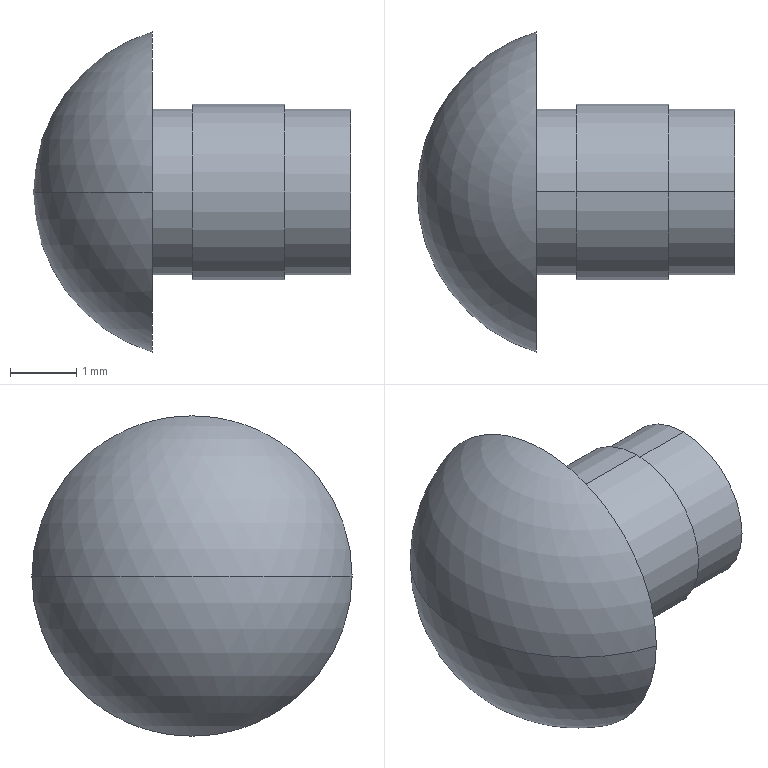Part | SolidWorks | features Boss 1, RevCut 1, Revolution 1 | 1 solid | 12 faces | box 4.8 x 4.84 x 4.84 mm | volume 35.188 mm3 | cylinder 6 | plane 4 | sphere 2 | commonest cylinder face diameters 2.5 x4 2.65 x2
STEP:
#1=CARTESIAN_POINT('',(3.8,0.,-1.25));
#2=VERTEX_POINT('',#1);
#3=CARTESIAN_POINT('',(3.8,0.,1.25));
#4=VERTEX_POINT('',#3);
#5=CARTESIAN_POINT('',(3.8,0.,0.));
#6=DIRECTION('',(1.,0.,0.));
#7=DIRECTION('',(0.,0.,-1.));
#8=AXIS2_PLACEMENT_3D('',#5,#6,#7);
#9=CIRCLE('',#8,1.25);
#10=EDGE_CURVE('',#2,#4,#9,.T.);
#11=ORIENTED_EDGE('',*,*,#10,.T.);
#12=CARTESIAN_POINT('',(4.8,0.,1.25));
#13=VERTEX_POINT('',#12);
#14=CARTESIAN_POINT('',(0.8134,0.,1.25));
#15=DIRECTION('',(1.,0.,0.));
#16=VECTOR('',#15,1000.);
#17=LINE('',#14,#16);
#18=EDGE_CURVE('',#4,#13,#17,.T.);
#19=ORIENTED_EDGE('',*,*,#18,.T.);
#20=CARTESIAN_POINT('',(4.8,0.,-1.25));
#21=VERTEX_POINT('',#20);
#22=CARTESIAN_POINT('',(4.8,0.,0.));
#23=DIRECTION('',(1.,0.,0.));
#24=DIRECTION('',(0.,0.,-1.));
#25=AXIS2_PLACEMENT_3D('',#22,#23,#24);
#26=CIRCLE('',#25,1.25);
#27=EDGE_CURVE('',#21,#13,#26,.T.);
#28=ORIENTED_EDGE('',*,*,#27,.F.);
#29=CARTESIAN_POINT('',(0.8134,0.,-1.25));
#30=DIRECTION('',(1.,0.,0.));
#31=VECTOR('',#30,1000.);
#32=LINE('',#29,#31);
#33=EDGE_CURVE('',#2,#21,#32,.T.);
#34=ORIENTED_EDGE('',*,*,#33,.F.);
#35=EDGE_LOOP('',(#11,#19,#28,#34));
#36=FACE_OUTER_BOUND('',#35,.T.);
#37=CARTESIAN_POINT('',(0.8134,0.,0.));
#38=DIRECTION('',(1.,0.,0.));
#39=DIRECTION('',(0.,0.,-1.));
#40=AXIS2_PLACEMENT_3D('',#37,#38,#39);
#41=CYLINDRICAL_SURFACE('',#40,1.25);
#42=ADVANCED_FACE('',(#36),#41,.T.);
#43=CARTESIAN_POINT('',(2.4,0.,-1.325));
#44=VERTEX_POINT('',#43);
#45=CARTESIAN_POINT('',(2.4,0.,1.325));
#46=VERTEX_POINT('',#45);
#47=CARTESIAN_POINT('',(2.4,0.,0.));
#48=DIRECTION('',(1.,0.,0.));
#49=DIRECTION('',(0.,0.,1.));
#50=AXIS2_PLACEMENT_3D('',#47,#48,#49);
#51=CIRCLE('',#50,1.325);
#52=EDGE_CURVE('',#44,#46,#51,.T.);
#53=ORIENTED_EDGE('',*,*,#52,.T.);
#54=CARTESIAN_POINT('',(3.8,0.,1.325));
#55=VERTEX_POINT('',#54);
#56=CARTESIAN_POINT('',(-1.948,0.,1.325));
#57=DIRECTION('',(1.,0.,0.));
#58=VECTOR('',#57,1000.);
#59=LINE('',#56,#58);
#60=EDGE_CURVE('',#46,#55,#59,.T.);
#61=ORIENTED_EDGE('',*,*,#60,.T.);
#62=CARTESIAN_POINT('',(3.8,0.,-1.325));
#63=VERTEX_POINT('',#62);
#64=CARTESIAN_POINT('',(3.8,0.,0.));
#65=DIRECTION('',(1.,0.,0.));
#66=DIRECTION('',(0.,0.,1.));
#67=AXIS2_PLACEMENT_3D('',#64,#65,#66);
#68=CIRCLE('',#67,1.325);
#69=EDGE_CURVE('',#63,#55,#68,.T.);
#70=ORIENTED_EDGE('',*,*,#69,.F.);
#71=CARTESIAN_POINT('',(-1.948,0.,-1.325));
#72=DIRECTION('',(1.,0.,0.));
#73=VECTOR('',#72,1000.);
#74=LINE('',#71,#73);
#75=EDGE_CURVE('',#44,#63,#74,.T.);
#76=ORIENTED_EDGE('',*,*,#75,.F.);
#77=EDGE_LOOP('',(#53,#61,#70,#76));
#78=FACE_OUTER_BOUND('',#77,.T.);
#79=CARTESIAN_POINT('',(-1.948,0.,0.));
#80=DIRECTION('',(1.,0.,0.));
#81=DIRECTION('',(0.,0.,-1.));
#82=AXIS2_PLACEMENT_3D('',#79,#80,#81);
#83=CYLINDRICAL_SURFACE('',#82,1.325);
#84=ADVANCED_FACE('',(#78),#83,.T.);
#85=CARTESIAN_POINT('',(1.8,2.42,0.));
#86=VERTEX_POINT('',#85);
#87=CARTESIAN_POINT('',(1.8,-2.42,0.));
#88=VERTEX_POINT('',#87);
#89=CARTESIAN_POINT('',(1.8,0.,0.));
#90=DIRECTION('',(-1.,0.,0.));
#91=DIRECTION('',(0.,0.,1.));
#92=AXIS2_PLACEMENT_3D('',#89,#90,#91);
#93=CIRCLE('',#92,2.42);
#94=EDGE_CURVE('',#86,#88,#93,.T.);
#95=ORIENTED_EDGE('',*,*,#94,.T.);
#96=CARTESIAN_POINT('',(0.,0.,0.));
#97=VERTEX_POINT('',#96);
#98=CARTESIAN_POINT('',(2.527,0.,0.));
#99=DIRECTION('',(0.,0.,-1.));
#100=DIRECTION('',(0.,1.,0.));
#101=AXIS2_PLACEMENT_3D('',#98,#99,#100);
#102=CIRCLE('',#101,2.527);
#103=EDGE_CURVE('',#88,#97,#102,.T.);
#104=ORIENTED_EDGE('',*,*,#103,.T.);
#105=CARTESIAN_POINT('',(2.527,0.,0.));
#106=DIRECTION('',(0.,0.,1.));
#107=DIRECTION('',(1.,0.,0.));
#108=AXIS2_PLACEMENT_3D('',#105,#106,#107);
#109=CIRCLE('',#108,2.527);
#110=EDGE_CURVE('',#86,#97,#109,.T.);
#111=ORIENTED_EDGE('',*,*,#110,.F.);
#112=EDGE_LOOP('',(#95,#104,#111));
#113=FACE_OUTER_BOUND('',#112,.T.);
#114=CARTESIAN_POINT('',(2.527,0.,0.));
#115=DIRECTION('',(0.,0.,-1.));
#116=DIRECTION('',(0.,1.,0.));
#117=AXIS2_PLACEMENT_3D('',#114,#115,#116);
#118=SPHERICAL_SURFACE('',#117,2.527);
#119=ADVANCED_FACE('',(#113),#118,.T.);
#120=CARTESIAN_POINT('',(2.4,0.,1.25));
#121=VERTEX_POINT('',#120);
#122=CARTESIAN_POINT('',(2.4,0.,-1.25));
#123=VERTEX_POINT('',#122);
#124=CARTESIAN_POINT('',(2.4,0.,0.));
#125=DIRECTION('',(-1.,0.,0.));
#126=DIRECTION('',(0.,0.,1.));
#127=AXIS2_PLACEMENT_3D('',#124,#125,#126);
#128=CIRCLE('',#127,1.25);
#129=EDGE_CURVE('',#121,#123,#128,.T.);
#130=ORIENTED_EDGE('',*,*,#129,.T.);
#131=CARTESIAN_POINT('',(1.8,0.,-1.25));
#132=VERTEX_POINT('',#131);
#133=CARTESIAN_POINT('',(-21.424,0.,-1.25));
#134=DIRECTION('',(-1.,0.,0.));
#135=VECTOR('',#134,1000.);
#136=LINE('',#133,#135);
#137=EDGE_CURVE('',#123,#132,#136,.T.);
#138=ORIENTED_EDGE('',*,*,#137,.T.);
#139=CARTESIAN_POINT('',(1.8,0.,1.25));
#140=VERTEX_POINT('',#139);
#141=CARTESIAN_POINT('',(1.8,0.,0.));
#142=DIRECTION('',(-1.,0.,0.));
#143=DIRECTION('',(0.,0.,1.));
#144=AXIS2_PLACEMENT_3D('',#141,#142,#143);
#145=CIRCLE('',#144,1.25);
#146=EDGE_CURVE('',#140,#132,#145,.T.);
#147=ORIENTED_EDGE('',*,*,#146,.F.);
#148=CARTESIAN_POINT('',(-21.424,0.,1.25));
#149=DIRECTION('',(-1.,0.,0.));
#150=VECTOR('',#149,1000.);
#151=LINE('',#148,#150);
#152=EDGE_CURVE('',#121,#140,#151,.T.);
#153=ORIENTED_EDGE('',*,*,#152,.F.);
#154=EDGE_LOOP('',(#130,#138,#147,#153));
#155=FACE_OUTER_BOUND('',#154,.T.);
#156=CARTESIAN_POINT('',(-21.424,0.,0.));
#157=DIRECTION('',(-1.,0.,0.));
#158=DIRECTION('',(0.,0.,1.));
#159=AXIS2_PLACEMENT_3D('',#156,#157,#158);
#160=CYLINDRICAL_SURFACE('',#159,1.25);
#161=ADVANCED_FACE('',(#155),#160,.T.);
#162=ORIENTED_EDGE('',*,*,#137,.F.);
#163=CARTESIAN_POINT('',(2.4,0.,0.));
#164=DIRECTION('',(-1.,0.,0.));
#165=DIRECTION('',(0.,0.,1.));
#166=AXIS2_PLACEMENT_3D('',#163,#164,#165);
#167=CIRCLE('',#166,1.25);
#168=EDGE_CURVE('',#123,#121,#167,.T.);
#169=ORIENTED_EDGE('',*,*,#168,.T.);
#170=ORIENTED_EDGE('',*,*,#152,.T.);
#171=CARTESIAN_POINT('',(1.8,0.,0.));
#172=DIRECTION('',(-1.,0.,0.));
#173=DIRECTION('',(0.,0.,1.));
#174=AXIS2_PLACEMENT_3D('',#171,#172,#173);
#175=CIRCLE('',#174,1.25);
#176=EDGE_CURVE('',#132,#140,#175,.T.);
#177=ORIENTED_EDGE('',*,*,#176,.F.);
#178=EDGE_LOOP('',(#162,#169,#170,#177));
#179=FACE_OUTER_BOUND('',#178,.T.);
#180=CARTESIAN_POINT('',(-21.424,0.,0.));
#181=DIRECTION('',(-1.,0.,0.));
#182=DIRECTION('',(0.,0.,1.));
#183=AXIS2_PLACEMENT_3D('',#180,#181,#182);
#184=CYLINDRICAL_SURFACE('',#183,1.25);
#185=ADVANCED_FACE('',(#179),#184,.T.);
#186=ORIENTED_EDGE('',*,*,#94,.F.);
#187=CARTESIAN_POINT('',(1.8,0.,0.));
#188=DIRECTION('',(-1.,0.,0.));
#189=DIRECTION('',(0.,0.,1.));
#190=AXIS2_PLACEMENT_3D('',#187,#188,#189);
#191=CIRCLE('',#190,2.42);
#192=EDGE_CURVE('',#88,#86,#191,.T.);
#193=ORIENTED_EDGE('',*,*,#192,.F.);
#194=EDGE_LOOP('',(#186,#193));
#195=FACE_OUTER_BOUND('',#194,.T.);
#196=ORIENTED_EDGE('',*,*,#146,.T.);
#197=ORIENTED_EDGE('',*,*,#176,.T.);
#198=EDGE_LOOP('',(#196,#197));
#199=FACE_BOUND('',#198,.T.);
#200=CARTESIAN_POINT('',(1.8,1.25,0.));
#201=DIRECTION('',(-1.,0.,0.));
#202=DIRECTION('',(0.,0.,1.));
#203=AXIS2_PLACEMENT_3D('',#200,#201,#202);
#204=PLANE('',#203);
#205=ADVANCED_FACE('',(#195,#199),#204,.F.);
#206=ORIENTED_EDGE('',*,*,#103,.F.);
#207=ORIENTED_EDGE('',*,*,#192,.T.);
#208=ORIENTED_EDGE('',*,*,#110,.T.);
#209=EDGE_LOOP('',(#206,#207,#208));
#210=FACE_OUTER_BOUND('',#209,.T.);
#211=CARTESIAN_POINT('',(2.527,0.,0.));
#212=DIRECTION('',(0.,0.,-1.));
#213=DIRECTION('',(0.,1.,0.));
#214=AXIS2_PLACEMENT_3D('',#211,#212,#213);
#215=SPHERICAL_SURFACE('',#214,2.527);
#216=ADVANCED_FACE('',(#210),#215,.T.);
#217=ORIENTED_EDGE('',*,*,#52,.F.);
#218=CARTESIAN_POINT('',(2.4,0.,0.));
#219=DIRECTION('',(1.,0.,0.));
#220=DIRECTION('',(0.,0.,1.));
#221=AXIS2_PLACEMENT_3D('',#218,#219,#220);
#222=CIRCLE('',#221,1.325);
#223=EDGE_CURVE('',#46,#44,#222,.T.);
#224=ORIENTED_EDGE('',*,*,#223,.F.);
#225=EDGE_LOOP('',(#217,#224));
#226=FACE_OUTER_BOUND('',#225,.T.);
#227=ORIENTED_EDGE('',*,*,#129,.F.);
#228=ORIENTED_EDGE('',*,*,#168,.F.);
#229=EDGE_LOOP('',(#227,#228));
#230=FACE_BOUND('',#229,.T.);
#231=CARTESIAN_POINT('',(2.4,1.25,0.));
#232=DIRECTION('',(-1.,0.,0.));
#233=DIRECTION('',(0.,0.,1.));
#234=AXIS2_PLACEMENT_3D('',#231,#232,#233);
#235=PLANE('',#234);
#236=ADVANCED_FACE('',(#226,#230),#235,.T.);
#237=ORIENTED_EDGE('',*,*,#60,.F.);
#238=ORIENTED_EDGE('',*,*,#223,.T.);
#239=ORIENTED_EDGE('',*,*,#75,.T.);
#240=CARTESIAN_POINT('',(3.8,0.,0.));
#241=DIRECTION('',(1.,0.,0.));
#242=DIRECTION('',(0.,0.,1.));
#243=AXIS2_PLACEMENT_3D('',#240,#241,#242);
#244=CIRCLE('',#243,1.325);
#245=EDGE_CURVE('',#55,#63,#244,.T.);
#246=ORIENTED_EDGE('',*,*,#245,.F.);
#247=EDGE_LOOP('',(#237,#238,#239,#246));
#248=FACE_OUTER_BOUND('',#247,.T.);
#249=CARTESIAN_POINT('',(-1.948,0.,0.));
#250=DIRECTION('',(1.,0.,0.));
#251=DIRECTION('',(0.,0.,-1.));
#252=AXIS2_PLACEMENT_3D('',#249,#250,#251);
#253=CYLINDRICAL_SURFACE('',#252,1.325);
#254=ADVANCED_FACE('',(#248),#253,.T.);
#255=ORIENTED_EDGE('',*,*,#18,.F.);
#256=CARTESIAN_POINT('',(3.8,0.,0.));
#257=DIRECTION('',(1.,0.,0.));
#258=DIRECTION('',(0.,0.,-1.));
#259=AXIS2_PLACEMENT_3D('',#256,#257,#258);
#260=CIRCLE('',#259,1.25);
#261=EDGE_CURVE('',#4,#2,#260,.T.);
#262=ORIENTED_EDGE('',*,*,#261,.T.);
#263=ORIENTED_EDGE('',*,*,#33,.T.);
#264=CARTESIAN_POINT('',(4.8,0.,0.));
#265=DIRECTION('',(1.,0.,0.));
#266=DIRECTION('',(0.,0.,-1.));
#267=AXIS2_PLACEMENT_3D('',#264,#265,#266);
#268=CIRCLE('',#267,1.25);
#269=EDGE_CURVE('',#13,#21,#268,.T.);
#270=ORIENTED_EDGE('',*,*,#269,.F.);
#271=EDGE_LOOP('',(#255,#262,#263,#270));
#272=FACE_OUTER_BOUND('',#271,.T.);
#273=CARTESIAN_POINT('',(0.8134,0.,0.));
#274=DIRECTION('',(1.,0.,0.));
#275=DIRECTION('',(0.,0.,-1.));
#276=AXIS2_PLACEMENT_3D('',#273,#274,#275);
#277=CYLINDRICAL_SURFACE('',#276,1.25);
#278=ADVANCED_FACE('',(#272),#277,.T.);
#279=ORIENTED_EDGE('',*,*,#69,.T.);
#280=ORIENTED_EDGE('',*,*,#245,.T.);
#281=EDGE_LOOP('',(#279,#280));
#282=FACE_OUTER_BOUND('',#281,.T.);
#283=ORIENTED_EDGE('',*,*,#10,.F.);
#284=ORIENTED_EDGE('',*,*,#261,.F.);
#285=EDGE_LOOP('',(#283,#284));
#286=FACE_BOUND('',#285,.T.);
#287=CARTESIAN_POINT('',(3.8,1.25,0.));
#288=DIRECTION('',(-1.,0.,0.));
#289=DIRECTION('',(0.,0.,1.));
#290=AXIS2_PLACEMENT_3D('',#287,#288,#289);
#291=PLANE('',#290);
#292=ADVANCED_FACE('',(#282,#286),#291,.F.);
#293=ORIENTED_EDGE('',*,*,#27,.T.);
#294=ORIENTED_EDGE('',*,*,#269,.T.);
#295=EDGE_LOOP('',(#293,#294));
#296=FACE_OUTER_BOUND('',#295,.T.);
#297=CARTESIAN_POINT('',(4.8,0.,0.));
#298=DIRECTION('',(-1.,0.,0.));
#299=DIRECTION('',(0.,0.,1.));
#300=AXIS2_PLACEMENT_3D('',#297,#298,#299);
#301=PLANE('',#300);
#302=ADVANCED_FACE('',(#296),#301,.F.);
#303=CLOSED_SHELL('',(#42,#84,#119,#161,#185,#205,#216,#236,#254,#278,#292,#302));
#304=MANIFOLD_SOLID_BREP('',#303);
#305=CARTESIAN_POINT('',(0.,0.,0.));
#306=DIRECTION('',(0.,0.,1.));
#307=DIRECTION('',(1.,0.,0.));
#308=AXIS2_PLACEMENT_3D('',#305,#306,#307);
#309=(LENGTH_UNIT()NAMED_UNIT(*)SI_UNIT(.MILLI.,.METRE.));
#310=UNCERTAINTY_MEASURE_WITH_UNIT(LENGTH_MEASURE(0.00001),#309,'','');
#311=(NAMED_UNIT(*)PLANE_ANGLE_UNIT()SI_UNIT($,.RADIAN.));
#312=(NAMED_UNIT(*)SI_UNIT($,.STERADIAN.)SOLID_ANGLE_UNIT());
#313=(GEOMETRIC_REPRESENTATION_CONTEXT(3)GLOBAL_UNCERTAINTY_ASSIGNED_CONTEXT((#310))GLOBAL_UNIT_ASSIGNED_CONTEXT((#309,#311,#312))REPRESENTATION_CONTEXT('',''));
#314=ADVANCED_BREP_SHAPE_REPRESENTATION('',(#304,#308),#313);